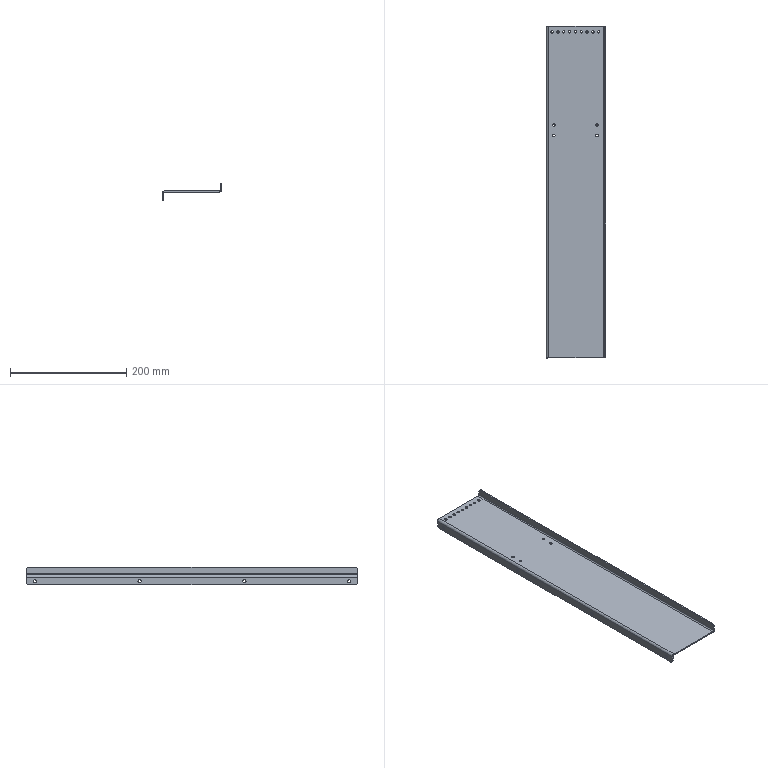Part | SolidWorks | features HoleWzd 3, Fillet 1, FlatPattern 1, SMBaseFlange 1, SheetMetal 1 | 1 solid | 60 faces | box 102 x 570 x 30 mm | volume 144671 mm3 | cylinder 42 | plane 18 | commonest cylinder face diameters 4.2 x26 5.5 x8 10 x4 4 x2 8 x2